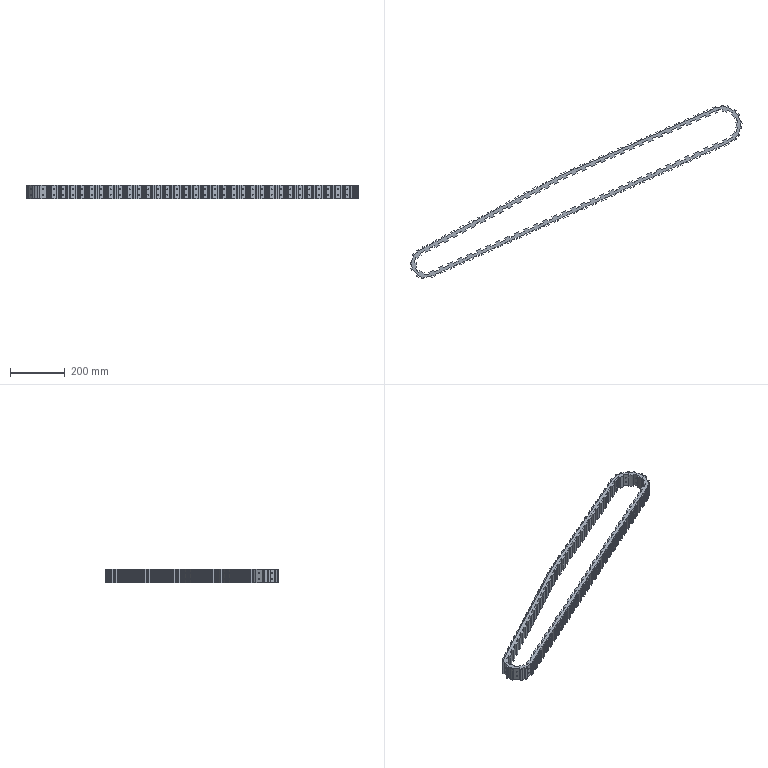Part | SolidWorks | features ICE 11, Extrusion 1 | 1 solid | 1176 faces | box 1216 x 635.295 x 50 mm | volume 2018846 mm3 | plane 860 | cylinder 316 | commonest cylinder face diameters 4 x284 144 x8 112.998 x7 69 x4 100 x4 134 x4